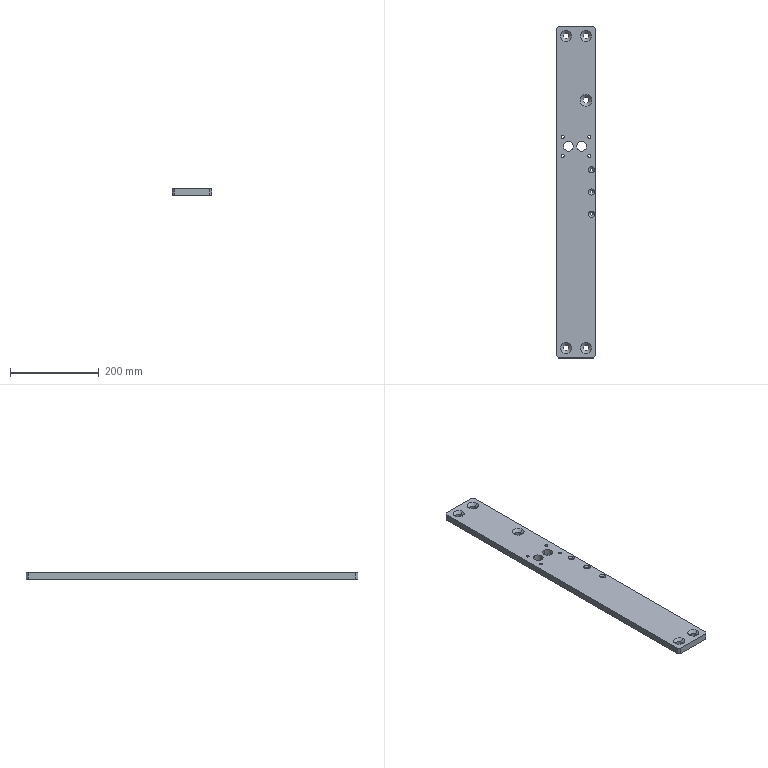Part | STEP file | 1 solid | 54 faces | box 90 x 748 x 15 mm | volume 978302 mm3 | cylinder 28 | cone 16 | plane 10 | commonest cylinder face diameters 6.8 x8 13 x8 6.6 x6 22 x4 13.5 x2